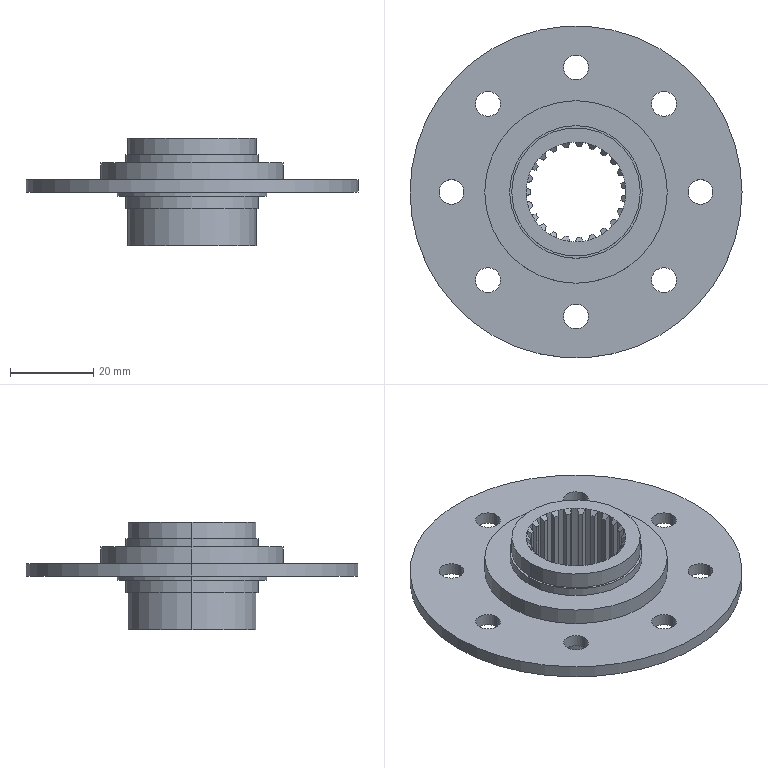Part | SolidWorks | features ICE 9, Extrusion 1, RevCut 1 | 1 solid | 178 faces | box 80 x 80 x 26 mm | volume 24406 mm3 | cylinder 77 | plane 54 | cone 47 | commonest cylinder face diameters 22 x24 24 x23 6 x16 31 x4 32 x4 36 x2